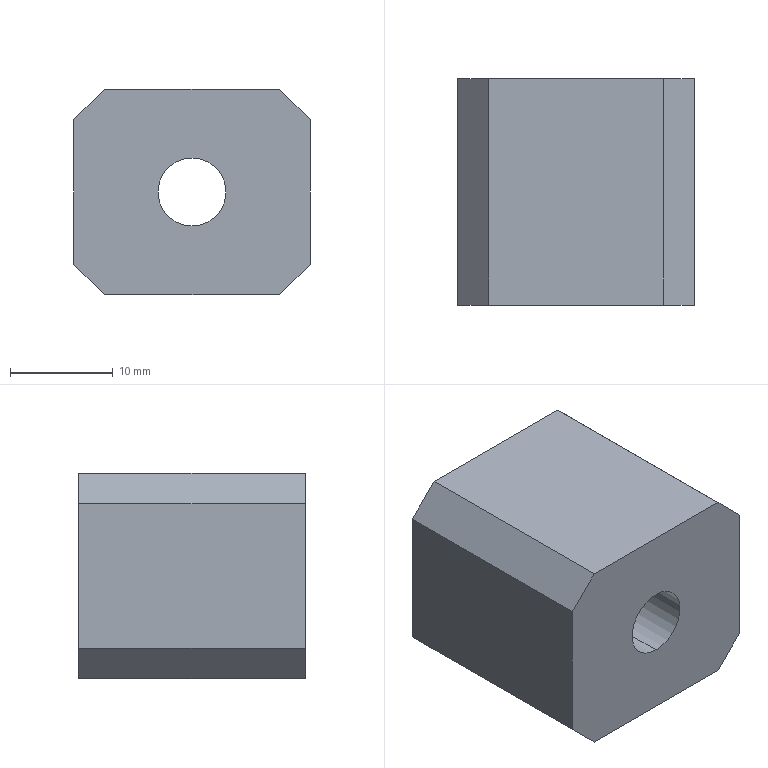Part | SolidWorks | features Chamfer 1, Extrusion 1, HoleWzd 1 | 1 solid | 15 faces | box 23 x 22 x 20 mm | volume 8558 mm3 | plane 11 | cylinder 4 | commonest cylinder face diameters 6.6 x2 11 x2
STEP:
#1=CARTESIAN_POINT('',(0.,15.2,4.5));
#2=VERTEX_POINT('',#1);
#3=CARTESIAN_POINT('',(0.,15.2,15.5));
#4=VERTEX_POINT('',#3);
#5=CARTESIAN_POINT('',(0.,15.2,10.));
#6=DIRECTION('',(0.,1.,0.));
#7=DIRECTION('',(0.,0.,1.));
#8=AXIS2_PLACEMENT_3D('',#5,#6,#7);
#9=CIRCLE('',#8,5.5);
#10=EDGE_CURVE('',#2,#4,#9,.T.);
#11=ORIENTED_EDGE('',*,*,#10,.F.);
#12=CARTESIAN_POINT('',(0.,22.,4.5));
#13=VERTEX_POINT('',#12);
#14=CARTESIAN_POINT('',(0.,22.,4.5));
#15=DIRECTION('',(0.,1.,0.));
#16=VECTOR('',#15,1000.);
#17=LINE('',#14,#16);
#18=EDGE_CURVE('',#2,#13,#17,.T.);
#19=ORIENTED_EDGE('',*,*,#18,.T.);
#20=CARTESIAN_POINT('',(0.,22.,15.5));
#21=VERTEX_POINT('',#20);
#22=CARTESIAN_POINT('',(0.,22.,10.));
#23=DIRECTION('',(0.,1.,0.));
#24=DIRECTION('',(0.,0.,1.));
#25=AXIS2_PLACEMENT_3D('',#22,#23,#24);
#26=CIRCLE('',#25,5.5);
#27=EDGE_CURVE('',#13,#21,#26,.T.);
#28=ORIENTED_EDGE('',*,*,#27,.T.);
#29=CARTESIAN_POINT('',(0.,22.,15.5));
#30=DIRECTION('',(0.,1.,0.));
#31=VECTOR('',#30,1000.);
#32=LINE('',#29,#31);
#33=EDGE_CURVE('',#4,#21,#32,.T.);
#34=ORIENTED_EDGE('',*,*,#33,.F.);
#35=EDGE_LOOP('',(#11,#19,#28,#34));
#36=FACE_OUTER_BOUND('',#35,.T.);
#37=CARTESIAN_POINT('',(0.,22.,10.));
#38=DIRECTION('',(0.,1.,0.));
#39=DIRECTION('',(0.,0.,1.));
#40=AXIS2_PLACEMENT_3D('',#37,#38,#39);
#41=CYLINDRICAL_SURFACE('',#40,5.5);
#42=ADVANCED_FACE('',(#36),#41,.F.);
#43=CARTESIAN_POINT('',(0.,0.,6.7));
#44=VERTEX_POINT('',#43);
#45=CARTESIAN_POINT('',(0.,0.,13.3));
#46=VERTEX_POINT('',#45);
#47=CARTESIAN_POINT('',(0.,0.,10.));
#48=DIRECTION('',(0.,1.,0.));
#49=DIRECTION('',(0.,0.,1.));
#50=AXIS2_PLACEMENT_3D('',#47,#48,#49);
#51=CIRCLE('',#50,3.3);
#52=EDGE_CURVE('',#44,#46,#51,.T.);
#53=ORIENTED_EDGE('',*,*,#52,.F.);
#54=CARTESIAN_POINT('',(0.,15.2,6.7));
#55=VERTEX_POINT('',#54);
#56=CARTESIAN_POINT('',(0.,22.,6.7));
#57=DIRECTION('',(0.,1.,0.));
#58=VECTOR('',#57,1000.);
#59=LINE('',#56,#58);
#60=EDGE_CURVE('',#44,#55,#59,.T.);
#61=ORIENTED_EDGE('',*,*,#60,.T.);
#62=CARTESIAN_POINT('',(0.,15.2,13.3));
#63=VERTEX_POINT('',#62);
#64=CARTESIAN_POINT('',(0.,15.2,10.));
#65=DIRECTION('',(0.,1.,0.));
#66=DIRECTION('',(0.,0.,1.));
#67=AXIS2_PLACEMENT_3D('',#64,#65,#66);
#68=CIRCLE('',#67,3.3);
#69=EDGE_CURVE('',#55,#63,#68,.T.);
#70=ORIENTED_EDGE('',*,*,#69,.T.);
#71=CARTESIAN_POINT('',(0.,22.,13.3));
#72=DIRECTION('',(0.,1.,0.));
#73=VECTOR('',#72,1000.);
#74=LINE('',#71,#73);
#75=EDGE_CURVE('',#46,#63,#74,.T.);
#76=ORIENTED_EDGE('',*,*,#75,.F.);
#77=EDGE_LOOP('',(#53,#61,#70,#76));
#78=FACE_OUTER_BOUND('',#77,.T.);
#79=CARTESIAN_POINT('',(0.,22.,10.));
#80=DIRECTION('',(0.,1.,0.));
#81=DIRECTION('',(0.,0.,1.));
#82=AXIS2_PLACEMENT_3D('',#79,#80,#81);
#83=CYLINDRICAL_SURFACE('',#82,3.3);
#84=ADVANCED_FACE('',(#78),#83,.F.);
#85=CARTESIAN_POINT('',(-11.5,22.,17.));
#86=VERTEX_POINT('',#85);
#87=CARTESIAN_POINT('',(-11.5,22.,3.));
#88=VERTEX_POINT('',#87);
#89=CARTESIAN_POINT('',(-11.5,22.,20.));
#90=DIRECTION('',(0.,0.,-1.));
#91=VECTOR('',#90,1000.);
#92=LINE('',#89,#91);
#93=EDGE_CURVE('',#86,#88,#92,.T.);
#94=ORIENTED_EDGE('',*,*,#93,.T.);
#95=CARTESIAN_POINT('',(-11.5,0.,3.));
#96=VERTEX_POINT('',#95);
#97=CARTESIAN_POINT('',(-11.5,22.,3.));
#98=DIRECTION('',(0.,-1.,0.));
#99=VECTOR('',#98,1000.);
#100=LINE('',#97,#99);
#101=EDGE_CURVE('',#88,#96,#100,.T.);
#102=ORIENTED_EDGE('',*,*,#101,.T.);
#103=CARTESIAN_POINT('',(-11.5,0.,17.));
#104=VERTEX_POINT('',#103);
#105=CARTESIAN_POINT('',(-11.5,0.,20.));
#106=DIRECTION('',(0.,0.,-1.));
#107=VECTOR('',#106,1000.);
#108=LINE('',#105,#107);
#109=EDGE_CURVE('',#104,#96,#108,.T.);
#110=ORIENTED_EDGE('',*,*,#109,.F.);
#111=CARTESIAN_POINT('',(-11.5,22.,17.));
#112=DIRECTION('',(0.,1.,0.));
#113=VECTOR('',#112,1000.);
#114=LINE('',#111,#113);
#115=EDGE_CURVE('',#104,#86,#114,.T.);
#116=ORIENTED_EDGE('',*,*,#115,.T.);
#117=EDGE_LOOP('',(#94,#102,#110,#116));
#118=FACE_OUTER_BOUND('',#117,.T.);
#119=CARTESIAN_POINT('',(-11.5,22.,20.));
#120=DIRECTION('',(1.,0.,0.));
#121=DIRECTION('',(0.,1.,0.));
#122=AXIS2_PLACEMENT_3D('',#119,#120,#121);
#123=PLANE('',#122);
#124=ADVANCED_FACE('',(#118),#123,.F.);
#125=CARTESIAN_POINT('',(0.,0.,10.));
#126=DIRECTION('',(0.,1.,0.));
#127=DIRECTION('',(0.,0.,1.));
#128=AXIS2_PLACEMENT_3D('',#125,#126,#127);
#129=CIRCLE('',#128,3.3);
#130=EDGE_CURVE('',#46,#44,#129,.T.);
#131=ORIENTED_EDGE('',*,*,#130,.T.);
#132=ORIENTED_EDGE('',*,*,#52,.T.);
#133=EDGE_LOOP('',(#131,#132));
#134=FACE_BOUND('',#133,.T.);
#135=ORIENTED_EDGE('',*,*,#109,.T.);
#136=CARTESIAN_POINT('',(-8.5,0.,0.));
#137=VERTEX_POINT('',#136);
#138=CARTESIAN_POINT('',(-11.5,0.,3.));
#139=DIRECTION('',(0.7071,0.,-0.7071));
#140=VECTOR('',#139,1000.);
#141=LINE('',#138,#140);
#142=EDGE_CURVE('',#96,#137,#141,.T.);
#143=ORIENTED_EDGE('',*,*,#142,.T.);
#144=CARTESIAN_POINT('',(8.5,0.,0.));
#145=VERTEX_POINT('',#144);
#146=CARTESIAN_POINT('',(-11.5,0.,0.));
#147=DIRECTION('',(1.,0.,0.));
#148=VECTOR('',#147,1000.);
#149=LINE('',#146,#148);
#150=EDGE_CURVE('',#137,#145,#149,.T.);
#151=ORIENTED_EDGE('',*,*,#150,.T.);
#152=CARTESIAN_POINT('',(11.5,0.,3.));
#153=VERTEX_POINT('',#152);
#154=CARTESIAN_POINT('',(11.5,0.,3.));
#155=DIRECTION('',(0.7071,0.,0.7071));
#156=VECTOR('',#155,1000.);
#157=LINE('',#154,#156);
#158=EDGE_CURVE('',#145,#153,#157,.T.);
#159=ORIENTED_EDGE('',*,*,#158,.T.);
#160=CARTESIAN_POINT('',(11.5,0.,17.));
#161=VERTEX_POINT('',#160);
#162=CARTESIAN_POINT('',(11.5,0.,20.));
#163=DIRECTION('',(0.,0.,-1.));
#164=VECTOR('',#163,1000.);
#165=LINE('',#162,#164);
#166=EDGE_CURVE('',#161,#153,#165,.T.);
#167=ORIENTED_EDGE('',*,*,#166,.F.);
#168=CARTESIAN_POINT('',(8.5,0.,20.));
#169=VERTEX_POINT('',#168);
#170=CARTESIAN_POINT('',(8.5,0.,20.));
#171=DIRECTION('',(-0.7071,0.,0.7071));
#172=VECTOR('',#171,1000.);
#173=LINE('',#170,#172);
#174=EDGE_CURVE('',#161,#169,#173,.T.);
#175=ORIENTED_EDGE('',*,*,#174,.T.);
#176=CARTESIAN_POINT('',(-8.5,0.,20.));
#177=VERTEX_POINT('',#176);
#178=CARTESIAN_POINT('',(-11.5,0.,20.));
#179=DIRECTION('',(1.,0.,0.));
#180=VECTOR('',#179,1000.);
#181=LINE('',#178,#180);
#182=EDGE_CURVE('',#177,#169,#181,.T.);
#183=ORIENTED_EDGE('',*,*,#182,.F.);
#184=CARTESIAN_POINT('',(-8.5,0.,20.));
#185=DIRECTION('',(-0.7071,0.,-0.7071));
#186=VECTOR('',#185,1000.);
#187=LINE('',#184,#186);
#188=EDGE_CURVE('',#177,#104,#187,.T.);
#189=ORIENTED_EDGE('',*,*,#188,.T.);
#190=EDGE_LOOP('',(#135,#143,#151,#159,#167,#175,#183,#189));
#191=FACE_OUTER_BOUND('',#190,.T.);
#192=CARTESIAN_POINT('',(-11.5,0.,20.));
#193=DIRECTION('',(0.,1.,0.));
#194=DIRECTION('',(0.,0.,1.));
#195=AXIS2_PLACEMENT_3D('',#192,#193,#194);
#196=PLANE('',#195);
#197=ADVANCED_FACE('',(#134,#191),#196,.F.);
#198=CARTESIAN_POINT('',(11.5,22.,17.));
#199=VERTEX_POINT('',#198);
#200=CARTESIAN_POINT('',(11.5,22.,3.));
#201=VERTEX_POINT('',#200);
#202=CARTESIAN_POINT('',(11.5,22.,20.));
#203=DIRECTION('',(0.,0.,-1.));
#204=VECTOR('',#203,1000.);
#205=LINE('',#202,#204);
#206=EDGE_CURVE('',#199,#201,#205,.T.);
#207=ORIENTED_EDGE('',*,*,#206,.F.);
#208=CARTESIAN_POINT('',(11.5,0.,17.));
#209=DIRECTION('',(0.,-1.,0.));
#210=VECTOR('',#209,1000.);
#211=LINE('',#208,#210);
#212=EDGE_CURVE('',#199,#161,#211,.T.);
#213=ORIENTED_EDGE('',*,*,#212,.T.);
#214=ORIENTED_EDGE('',*,*,#166,.T.);
#215=CARTESIAN_POINT('',(11.5,22.,3.));
#216=DIRECTION('',(0.,1.,0.));
#217=VECTOR('',#216,1000.);
#218=LINE('',#215,#217);
#219=EDGE_CURVE('',#153,#201,#218,.T.);
#220=ORIENTED_EDGE('',*,*,#219,.T.);
#221=EDGE_LOOP('',(#207,#213,#214,#220));
#222=FACE_OUTER_BOUND('',#221,.T.);
#223=CARTESIAN_POINT('',(11.5,22.,20.));
#224=DIRECTION('',(-1.,0.,0.));
#225=DIRECTION('',(0.,-1.,0.));
#226=AXIS2_PLACEMENT_3D('',#223,#224,#225);
#227=PLANE('',#226);
#228=ADVANCED_FACE('',(#222),#227,.F.);
#229=CARTESIAN_POINT('',(0.,22.,10.));
#230=DIRECTION('',(0.,1.,0.));
#231=DIRECTION('',(0.,0.,1.));
#232=AXIS2_PLACEMENT_3D('',#229,#230,#231);
#233=CIRCLE('',#232,5.5);
#234=EDGE_CURVE('',#21,#13,#233,.T.);
#235=ORIENTED_EDGE('',*,*,#234,.F.);
#236=ORIENTED_EDGE('',*,*,#27,.F.);
#237=EDGE_LOOP('',(#235,#236));
#238=FACE_BOUND('',#237,.T.);
#239=CARTESIAN_POINT('',(8.5,22.,0.));
#240=VERTEX_POINT('',#239);
#241=CARTESIAN_POINT('',(-8.5,22.,0.));
#242=VERTEX_POINT('',#241);
#243=CARTESIAN_POINT('',(-11.5,22.,0.));
#244=DIRECTION('',(-1.,0.,0.));
#245=VECTOR('',#244,1000.);
#246=LINE('',#243,#245);
#247=EDGE_CURVE('',#240,#242,#246,.T.);
#248=ORIENTED_EDGE('',*,*,#247,.T.);
#249=CARTESIAN_POINT('',(-11.5,22.,3.));
#250=DIRECTION('',(-0.7071,0.,0.7071));
#251=VECTOR('',#250,1000.);
#252=LINE('',#249,#251);
#253=EDGE_CURVE('',#242,#88,#252,.T.);
#254=ORIENTED_EDGE('',*,*,#253,.T.);
#255=ORIENTED_EDGE('',*,*,#93,.F.);
#256=CARTESIAN_POINT('',(-8.5,22.,20.));
#257=VERTEX_POINT('',#256);
#258=CARTESIAN_POINT('',(-8.5,22.,20.));
#259=DIRECTION('',(0.7071,0.,0.7071));
#260=VECTOR('',#259,1000.);
#261=LINE('',#258,#260);
#262=EDGE_CURVE('',#86,#257,#261,.T.);
#263=ORIENTED_EDGE('',*,*,#262,.T.);
#264=CARTESIAN_POINT('',(8.5,22.,20.));
#265=VERTEX_POINT('',#264);
#266=CARTESIAN_POINT('',(-11.5,22.,20.));
#267=DIRECTION('',(-1.,0.,0.));
#268=VECTOR('',#267,1000.);
#269=LINE('',#266,#268);
#270=EDGE_CURVE('',#265,#257,#269,.T.);
#271=ORIENTED_EDGE('',*,*,#270,.F.);
#272=CARTESIAN_POINT('',(8.5,22.,20.));
#273=DIRECTION('',(0.7071,0.,-0.7071));
#274=VECTOR('',#273,1000.);
#275=LINE('',#272,#274);
#276=EDGE_CURVE('',#265,#199,#275,.T.);
#277=ORIENTED_EDGE('',*,*,#276,.T.);
#278=ORIENTED_EDGE('',*,*,#206,.T.);
#279=CARTESIAN_POINT('',(11.5,22.,3.));
#280=DIRECTION('',(-0.7071,0.,-0.7071));
#281=VECTOR('',#280,1000.);
#282=LINE('',#279,#281);
#283=EDGE_CURVE('',#201,#240,#282,.T.);
#284=ORIENTED_EDGE('',*,*,#283,.T.);
#285=EDGE_LOOP('',(#248,#254,#255,#263,#271,#277,#278,#284));
#286=FACE_OUTER_BOUND('',#285,.T.);
#287=CARTESIAN_POINT('',(-11.5,22.,20.));
#288=DIRECTION('',(0.,-1.,0.));
#289=DIRECTION('',(0.,0.,-1.));
#290=AXIS2_PLACEMENT_3D('',#287,#288,#289);
#291=PLANE('',#290);
#292=ADVANCED_FACE('',(#238,#286),#291,.F.);
#293=ORIENTED_EDGE('',*,*,#270,.T.);
#294=CARTESIAN_POINT('',(-8.5,0.,20.));
#295=DIRECTION('',(0.,-1.,0.));
#296=VECTOR('',#295,1000.);
#297=LINE('',#294,#296);
#298=EDGE_CURVE('',#257,#177,#297,.T.);
#299=ORIENTED_EDGE('',*,*,#298,.T.);
#300=ORIENTED_EDGE('',*,*,#182,.T.);
#301=CARTESIAN_POINT('',(8.5,22.,20.));
#302=DIRECTION('',(0.,1.,0.));
#303=VECTOR('',#302,1000.);
#304=LINE('',#301,#303);
#305=EDGE_CURVE('',#169,#265,#304,.T.);
#306=ORIENTED_EDGE('',*,*,#305,.T.);
#307=EDGE_LOOP('',(#293,#299,#300,#306));
#308=FACE_OUTER_BOUND('',#307,.T.);
#309=CARTESIAN_POINT('',(0.,0.,20.));
#310=DIRECTION('',(0.,0.,1.));
#311=DIRECTION('',(1.,0.,0.));
#312=AXIS2_PLACEMENT_3D('',#309,#310,#311);
#313=PLANE('',#312);
#314=ADVANCED_FACE('',(#308),#313,.T.);
#315=ORIENTED_EDGE('',*,*,#150,.F.);
#316=CARTESIAN_POINT('',(-8.5,0.,0.));
#317=DIRECTION('',(0.,1.,0.));
#318=VECTOR('',#317,1000.);
#319=LINE('',#316,#318);
#320=EDGE_CURVE('',#137,#242,#319,.T.);
#321=ORIENTED_EDGE('',*,*,#320,.T.);
#322=ORIENTED_EDGE('',*,*,#247,.F.);
#323=CARTESIAN_POINT('',(8.5,0.,0.));
#324=DIRECTION('',(0.,-1.,0.));
#325=VECTOR('',#324,1000.);
#326=LINE('',#323,#325);
#327=EDGE_CURVE('',#240,#145,#326,.T.);
#328=ORIENTED_EDGE('',*,*,#327,.T.);
#329=EDGE_LOOP('',(#315,#321,#322,#328));
#330=FACE_OUTER_BOUND('',#329,.T.);
#331=CARTESIAN_POINT('',(0.,0.,0.));
#332=DIRECTION('',(0.,0.,1.));
#333=DIRECTION('',(1.,0.,0.));
#334=AXIS2_PLACEMENT_3D('',#331,#332,#333);
#335=PLANE('',#334);
#336=ADVANCED_FACE('',(#330),#335,.F.);
#337=ORIENTED_EDGE('',*,*,#60,.F.);
#338=ORIENTED_EDGE('',*,*,#130,.F.);
#339=ORIENTED_EDGE('',*,*,#75,.T.);
#340=CARTESIAN_POINT('',(0.,15.2,10.));
#341=DIRECTION('',(0.,1.,0.));
#342=DIRECTION('',(0.,0.,1.));
#343=AXIS2_PLACEMENT_3D('',#340,#341,#342);
#344=CIRCLE('',#343,3.3);
#345=EDGE_CURVE('',#63,#55,#344,.T.);
#346=ORIENTED_EDGE('',*,*,#345,.T.);
#347=EDGE_LOOP('',(#337,#338,#339,#346));
#348=FACE_OUTER_BOUND('',#347,.T.);
#349=CARTESIAN_POINT('',(0.,22.,10.));
#350=DIRECTION('',(0.,1.,0.));
#351=DIRECTION('',(0.,0.,1.));
#352=AXIS2_PLACEMENT_3D('',#349,#350,#351);
#353=CYLINDRICAL_SURFACE('',#352,3.3);
#354=ADVANCED_FACE('',(#348),#353,.F.);
#355=ORIENTED_EDGE('',*,*,#345,.F.);
#356=ORIENTED_EDGE('',*,*,#69,.F.);
#357=EDGE_LOOP('',(#355,#356));
#358=FACE_BOUND('',#357,.T.);
#359=CARTESIAN_POINT('',(0.,15.2,10.));
#360=DIRECTION('',(0.,1.,0.));
#361=DIRECTION('',(0.,0.,1.));
#362=AXIS2_PLACEMENT_3D('',#359,#360,#361);
#363=CIRCLE('',#362,5.5);
#364=EDGE_CURVE('',#4,#2,#363,.T.);
#365=ORIENTED_EDGE('',*,*,#364,.T.);
#366=ORIENTED_EDGE('',*,*,#10,.T.);
#367=EDGE_LOOP('',(#365,#366));
#368=FACE_OUTER_BOUND('',#367,.T.);
#369=CARTESIAN_POINT('',(3.3,15.2,10.));
#370=DIRECTION('',(0.,-1.,0.));
#371=DIRECTION('',(0.,0.,-1.));
#372=AXIS2_PLACEMENT_3D('',#369,#370,#371);
#373=PLANE('',#372);
#374=ADVANCED_FACE('',(#358,#368),#373,.F.);
#375=ORIENTED_EDGE('',*,*,#18,.F.);
#376=ORIENTED_EDGE('',*,*,#364,.F.);
#377=ORIENTED_EDGE('',*,*,#33,.T.);
#378=ORIENTED_EDGE('',*,*,#234,.T.);
#379=EDGE_LOOP('',(#375,#376,#377,#378));
#380=FACE_OUTER_BOUND('',#379,.T.);
#381=CARTESIAN_POINT('',(0.,22.,10.));
#382=DIRECTION('',(0.,1.,0.));
#383=DIRECTION('',(0.,0.,1.));
#384=AXIS2_PLACEMENT_3D('',#381,#382,#383);
#385=CYLINDRICAL_SURFACE('',#384,5.5);
#386=ADVANCED_FACE('',(#380),#385,.F.);
#387=ORIENTED_EDGE('',*,*,#253,.F.);
#388=ORIENTED_EDGE('',*,*,#320,.F.);
#389=ORIENTED_EDGE('',*,*,#142,.F.);
#390=ORIENTED_EDGE('',*,*,#101,.F.);
#391=EDGE_LOOP('',(#387,#388,#389,#390));
#392=FACE_OUTER_BOUND('',#391,.T.);
#393=CARTESIAN_POINT('',(-11.5,22.,3.));
#394=DIRECTION('',(0.7071,0.,0.7071));
#395=DIRECTION('',(0.,-1.,0.));
#396=AXIS2_PLACEMENT_3D('',#393,#394,#395);
#397=PLANE('',#396);
#398=ADVANCED_FACE('',(#392),#397,.F.);
#399=ORIENTED_EDGE('',*,*,#262,.F.);
#400=ORIENTED_EDGE('',*,*,#115,.F.);
#401=ORIENTED_EDGE('',*,*,#188,.F.);
#402=ORIENTED_EDGE('',*,*,#298,.F.);
#403=EDGE_LOOP('',(#399,#400,#401,#402));
#404=FACE_OUTER_BOUND('',#403,.T.);
#405=CARTESIAN_POINT('',(-8.5,0.,20.));
#406=DIRECTION('',(-0.7071,0.,0.7071));
#407=DIRECTION('',(0.,1.,0.));
#408=AXIS2_PLACEMENT_3D('',#405,#406,#407);
#409=PLANE('',#408);
#410=ADVANCED_FACE('',(#404),#409,.T.);
#411=ORIENTED_EDGE('',*,*,#174,.F.);
#412=ORIENTED_EDGE('',*,*,#212,.F.);
#413=ORIENTED_EDGE('',*,*,#276,.F.);
#414=ORIENTED_EDGE('',*,*,#305,.F.);
#415=EDGE_LOOP('',(#411,#412,#413,#414));
#416=FACE_OUTER_BOUND('',#415,.T.);
#417=CARTESIAN_POINT('',(8.5,0.,20.));
#418=DIRECTION('',(0.7071,0.,0.7071));
#419=DIRECTION('',(0.,-1.,0.));
#420=AXIS2_PLACEMENT_3D('',#417,#418,#419);
#421=PLANE('',#420);
#422=ADVANCED_FACE('',(#416),#421,.T.);
#423=ORIENTED_EDGE('',*,*,#158,.F.);
#424=ORIENTED_EDGE('',*,*,#327,.F.);
#425=ORIENTED_EDGE('',*,*,#283,.F.);
#426=ORIENTED_EDGE('',*,*,#219,.F.);
#427=EDGE_LOOP('',(#423,#424,#425,#426));
#428=FACE_OUTER_BOUND('',#427,.T.);
#429=CARTESIAN_POINT('',(11.5,22.,3.));
#430=DIRECTION('',(-0.7071,0.,0.7071));
#431=DIRECTION('',(0.,1.,0.));
#432=AXIS2_PLACEMENT_3D('',#429,#430,#431);
#433=PLANE('',#432);
#434=ADVANCED_FACE('',(#428),#433,.F.);
#435=CLOSED_SHELL('',(#42,#84,#124,#197,#228,#292,#314,#336,#354,#374,#386,#398,#410,#422,#434));
#436=MANIFOLD_SOLID_BREP('',#435);
#437=CARTESIAN_POINT('',(0.,0.,0.));
#438=DIRECTION('',(0.,0.,1.));
#439=DIRECTION('',(1.,0.,0.));
#440=AXIS2_PLACEMENT_3D('',#437,#438,#439);
#441=(LENGTH_UNIT()NAMED_UNIT(*)SI_UNIT(.MILLI.,.METRE.));
#442=UNCERTAINTY_MEASURE_WITH_UNIT(LENGTH_MEASURE(0.00001),#441,'','');
#443=(NAMED_UNIT(*)PLANE_ANGLE_UNIT()SI_UNIT($,.RADIAN.));
#444=(NAMED_UNIT(*)SI_UNIT($,.STERADIAN.)SOLID_ANGLE_UNIT());
#445=(GEOMETRIC_REPRESENTATION_CONTEXT(3)GLOBAL_UNCERTAINTY_ASSIGNED_CONTEXT((#442))GLOBAL_UNIT_ASSIGNED_CONTEXT((#441,#443,#444))REPRESENTATION_CONTEXT('',''));
#446=ADVANCED_BREP_SHAPE_REPRESENTATION('',(#436,#440),#445);